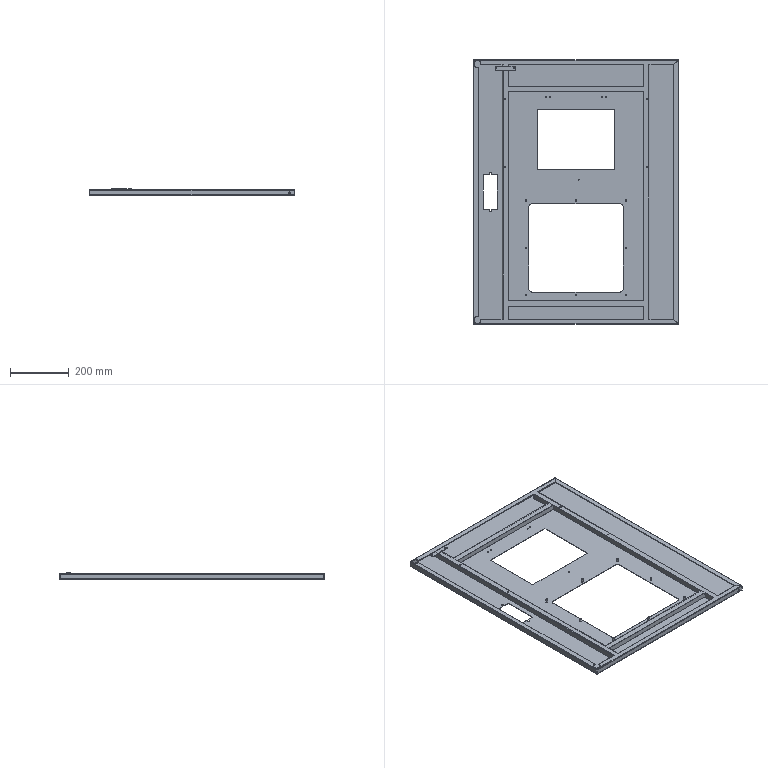Part | STEP file | ND22021-MA-C-111-BJ | 1 solid | 195 faces | box 700 x 900 x 22 mm | volume 1108313 mm3 | plane 103 | cylinder 76 | spline 16 | commonest cylinder face diameters 6 x20 3.3 x10 1.473 x8 4.2 x8 4.473 x8 4 x6